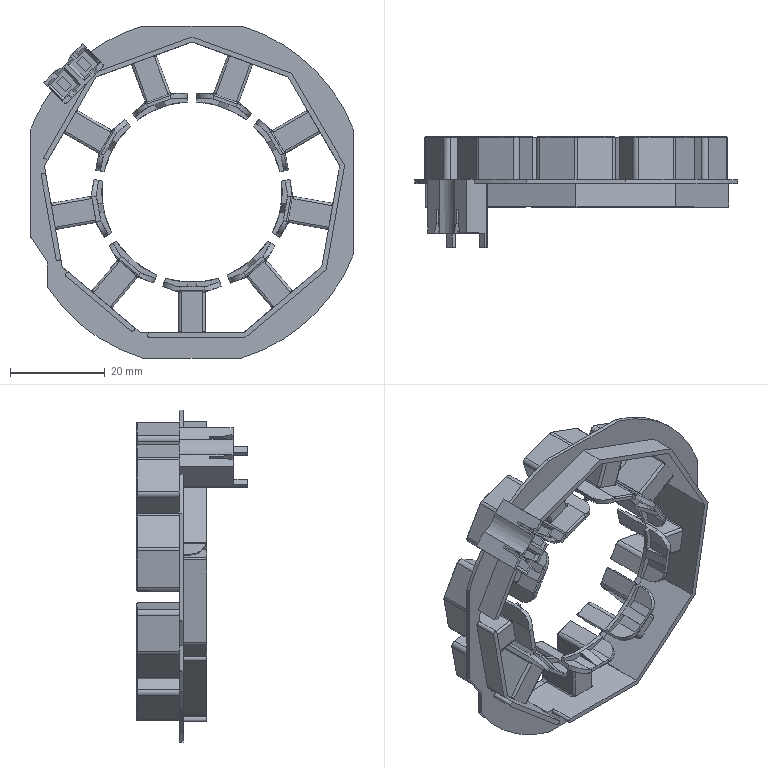Part | STEP file | XIAHUTAO_29_1 | 1 solid | 864 faces | box 68 x 23.3 x 70 mm | volume 5989 mm3 | plane 491 | cylinder 221 | cone 99 | torus 53 | commonest cylinder face diameters 0.4 x45 1.2 x45 2 x45 1 x44 7 x18 0.6 x9